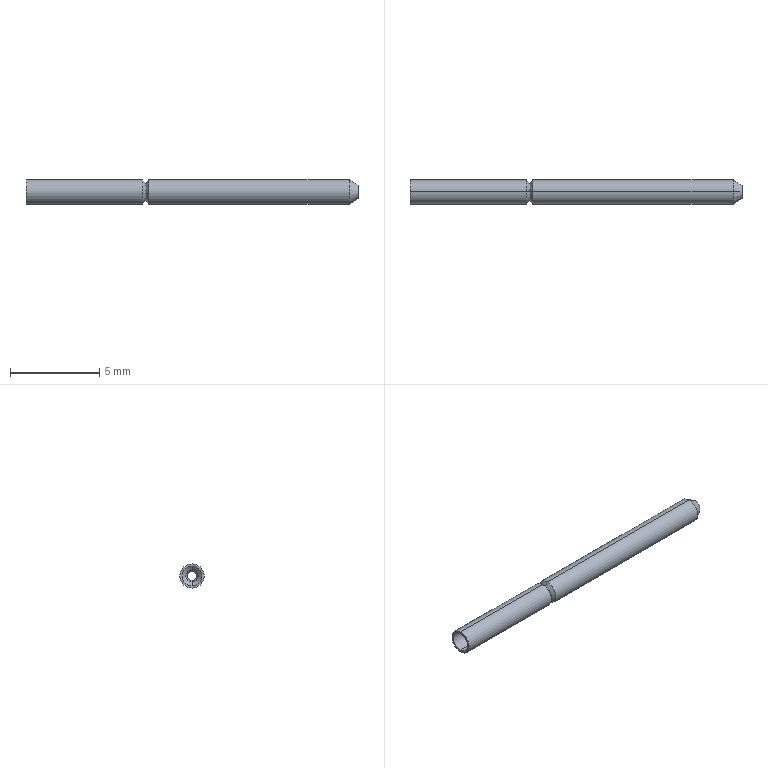Part | STEP file | Barrel_NP604_B | 1 solid | 22 faces | box 18.6 x 1.36 x 1.36 mm | volume 8.939 mm3 | cone 12 | cylinder 8 | plane 2 | commonest cylinder face diameters 1.11 x4 1.36 x4
STEP:
#1=CARTESIAN_POINT('',(6.7,0.,0.4714));
#2=VERTEX_POINT('',#1);
#3=CARTESIAN_POINT('',(6.7,0.,-0.4714));
#4=VERTEX_POINT('',#3);
#5=CARTESIAN_POINT('',(6.7,0.,0.));
#6=DIRECTION('',(-1.,0.,0.));
#7=DIRECTION('',(0.,0.,1.));
#8=AXIS2_PLACEMENT_3D('',#5,#6,#7);
#9=CIRCLE('',#8,0.4714);
#10=EDGE_CURVE('',#2,#4,#9,.T.);
#11=ORIENTED_EDGE('',*,*,#10,.T.);
#12=CARTESIAN_POINT('',(6.525,0.,-0.68));
#13=VERTEX_POINT('',#12);
#14=CARTESIAN_POINT('',(6.7,0.,-0.4714));
#15=DIRECTION('',(-0.6428,0.,-0.766));
#16=VECTOR('',#15,1000.);
#17=LINE('',#14,#16);
#18=EDGE_CURVE('',#4,#13,#17,.T.);
#19=ORIENTED_EDGE('',*,*,#18,.T.);
#20=CARTESIAN_POINT('',(6.525,0.,0.68));
#21=VERTEX_POINT('',#20);
#22=CARTESIAN_POINT('',(6.525,0.,0.));
#23=DIRECTION('',(-1.,0.,0.));
#24=DIRECTION('',(0.,0.,1.));
#25=AXIS2_PLACEMENT_3D('',#22,#23,#24);
#26=CIRCLE('',#25,0.68);
#27=EDGE_CURVE('',#21,#13,#26,.T.);
#28=ORIENTED_EDGE('',*,*,#27,.F.);
#29=CARTESIAN_POINT('',(6.7,0.,0.4714));
#30=DIRECTION('',(-0.6428,0.,0.766));
#31=VECTOR('',#30,1000.);
#32=LINE('',#29,#31);
#33=EDGE_CURVE('',#2,#21,#32,.T.);
#34=ORIENTED_EDGE('',*,*,#33,.F.);
#35=EDGE_LOOP('',(#11,#19,#28,#34));
#36=FACE_OUTER_BOUND('',#35,.T.);
#37=CARTESIAN_POINT('',(6.7,0.,0.));
#38=DIRECTION('',(-1.,0.,0.));
#39=DIRECTION('',(0.,0.,1.));
#40=AXIS2_PLACEMENT_3D('',#37,#38,#39);
#41=CONICAL_SURFACE('',#40,0.4714,0.8727);
#42=ADVANCED_FACE('',(#36),#41,.T.);
#43=ORIENTED_EDGE('',*,*,#10,.F.);
#44=CARTESIAN_POINT('',(6.875,0.,0.68));
#45=VERTEX_POINT('',#44);
#46=CARTESIAN_POINT('',(6.875,0.,0.68));
#47=DIRECTION('',(0.6428,0.,0.766));
#48=VECTOR('',#47,1000.);
#49=LINE('',#46,#48);
#50=EDGE_CURVE('',#2,#45,#49,.T.);
#51=ORIENTED_EDGE('',*,*,#50,.T.);
#52=CARTESIAN_POINT('',(6.875,0.,-0.68));
#53=VERTEX_POINT('',#52);
#54=CARTESIAN_POINT('',(6.875,0.,0.));
#55=DIRECTION('',(-1.,0.,0.));
#56=DIRECTION('',(0.,0.,1.));
#57=AXIS2_PLACEMENT_3D('',#54,#55,#56);
#58=CIRCLE('',#57,0.68);
#59=EDGE_CURVE('',#45,#53,#58,.T.);
#60=ORIENTED_EDGE('',*,*,#59,.T.);
#61=CARTESIAN_POINT('',(6.875,0.,-0.68));
#62=DIRECTION('',(0.6428,0.,-0.766));
#63=VECTOR('',#62,1000.);
#64=LINE('',#61,#63);
#65=EDGE_CURVE('',#4,#53,#64,.T.);
#66=ORIENTED_EDGE('',*,*,#65,.F.);
#67=EDGE_LOOP('',(#43,#51,#60,#66));
#68=FACE_OUTER_BOUND('',#67,.T.);
#69=CARTESIAN_POINT('',(6.875,0.,0.));
#70=DIRECTION('',(1.,0.,0.));
#71=DIRECTION('',(0.,0.,-1.));
#72=AXIS2_PLACEMENT_3D('',#69,#70,#71);
#73=CONICAL_SURFACE('',#72,0.68,0.8727);
#74=ADVANCED_FACE('',(#68),#73,.T.);
#75=CARTESIAN_POINT('',(18.1,0.,0.68));
#76=VERTEX_POINT('',#75);
#77=CARTESIAN_POINT('',(18.1,0.,-0.68));
#78=VERTEX_POINT('',#77);
#79=CARTESIAN_POINT('',(18.1,0.,0.));
#80=DIRECTION('',(-1.,0.,0.));
#81=DIRECTION('',(0.,0.,1.));
#82=AXIS2_PLACEMENT_3D('',#79,#80,#81);
#83=CIRCLE('',#82,0.68);
#84=EDGE_CURVE('',#76,#78,#83,.T.);
#85=ORIENTED_EDGE('',*,*,#84,.T.);
#86=CARTESIAN_POINT('',(18.6,0.,-0.68));
#87=DIRECTION('',(-1.,0.,0.));
#88=VECTOR('',#87,1000.);
#89=LINE('',#86,#88);
#90=EDGE_CURVE('',#78,#53,#89,.T.);
#91=ORIENTED_EDGE('',*,*,#90,.T.);
#92=ORIENTED_EDGE('',*,*,#59,.F.);
#93=CARTESIAN_POINT('',(18.6,0.,0.68));
#94=DIRECTION('',(-1.,0.,0.));
#95=VECTOR('',#94,1000.);
#96=LINE('',#93,#95);
#97=EDGE_CURVE('',#76,#45,#96,.T.);
#98=ORIENTED_EDGE('',*,*,#97,.F.);
#99=EDGE_LOOP('',(#85,#91,#92,#98));
#100=FACE_OUTER_BOUND('',#99,.T.);
#101=CARTESIAN_POINT('',(18.6,0.,0.));
#102=DIRECTION('',(-1.,0.,0.));
#103=DIRECTION('',(0.,0.,1.));
#104=AXIS2_PLACEMENT_3D('',#101,#102,#103);
#105=CYLINDRICAL_SURFACE('',#104,0.68);
#106=ADVANCED_FACE('',(#100),#105,.T.);
#107=CARTESIAN_POINT('',(18.6,0.,0.375));
#108=VERTEX_POINT('',#107);
#109=CARTESIAN_POINT('',(18.6,0.,-0.375));
#110=VERTEX_POINT('',#109);
#111=CARTESIAN_POINT('',(18.6,0.,0.));
#112=DIRECTION('',(-1.,0.,0.));
#113=DIRECTION('',(0.,0.,1.));
#114=AXIS2_PLACEMENT_3D('',#111,#112,#113);
#115=CIRCLE('',#114,0.375);
#116=EDGE_CURVE('',#108,#110,#115,.T.);
#117=ORIENTED_EDGE('',*,*,#116,.T.);
#118=CARTESIAN_POINT('',(18.6,0.,-0.375));
#119=DIRECTION('',(-0.8537,0.,-0.5208));
#120=VECTOR('',#119,1000.);
#121=LINE('',#118,#120);
#122=EDGE_CURVE('',#110,#78,#121,.T.);
#123=ORIENTED_EDGE('',*,*,#122,.T.);
#124=ORIENTED_EDGE('',*,*,#84,.F.);
#125=CARTESIAN_POINT('',(18.6,0.,0.375));
#126=DIRECTION('',(-0.8537,0.,0.5208));
#127=VECTOR('',#126,1000.);
#128=LINE('',#125,#127);
#129=EDGE_CURVE('',#108,#76,#128,.T.);
#130=ORIENTED_EDGE('',*,*,#129,.F.);
#131=EDGE_LOOP('',(#117,#123,#124,#130));
#132=FACE_OUTER_BOUND('',#131,.T.);
#133=CARTESIAN_POINT('',(18.6,0.,0.));
#134=DIRECTION('',(-1.,0.,0.));
#135=DIRECTION('',(0.,0.,1.));
#136=AXIS2_PLACEMENT_3D('',#133,#134,#135);
#137=CONICAL_SURFACE('',#136,0.375,0.5477);
#138=ADVANCED_FACE('',(#132),#137,.T.);
#139=CARTESIAN_POINT('',(18.6,0.,-0.25));
#140=VERTEX_POINT('',#139);
#141=CARTESIAN_POINT('',(18.6,0.,0.25));
#142=VERTEX_POINT('',#141);
#143=CARTESIAN_POINT('',(18.6,0.,0.));
#144=DIRECTION('',(-1.,0.,0.));
#145=DIRECTION('',(0.,0.,1.));
#146=AXIS2_PLACEMENT_3D('',#143,#144,#145);
#147=CIRCLE('',#146,0.25);
#148=EDGE_CURVE('',#140,#142,#147,.T.);
#149=ORIENTED_EDGE('',*,*,#148,.F.);
#150=CARTESIAN_POINT('',(18.1,0.,-0.555));
#151=VERTEX_POINT('',#150);
#152=CARTESIAN_POINT('',(18.1,0.,-0.555));
#153=DIRECTION('',(-0.8537,0.,-0.5208));
#154=VECTOR('',#153,1000.);
#155=LINE('',#152,#154);
#156=EDGE_CURVE('',#140,#151,#155,.T.);
#157=ORIENTED_EDGE('',*,*,#156,.T.);
#158=CARTESIAN_POINT('',(18.1,0.,0.555));
#159=VERTEX_POINT('',#158);
#160=CARTESIAN_POINT('',(18.1,0.,0.));
#161=DIRECTION('',(-1.,0.,0.));
#162=DIRECTION('',(0.,0.,1.));
#163=AXIS2_PLACEMENT_3D('',#160,#161,#162);
#164=CIRCLE('',#163,0.555);
#165=EDGE_CURVE('',#151,#159,#164,.T.);
#166=ORIENTED_EDGE('',*,*,#165,.T.);
#167=CARTESIAN_POINT('',(18.1,0.,0.555));
#168=DIRECTION('',(-0.8537,0.,0.5208));
#169=VECTOR('',#168,1000.);
#170=LINE('',#167,#169);
#171=EDGE_CURVE('',#142,#159,#170,.T.);
#172=ORIENTED_EDGE('',*,*,#171,.F.);
#173=EDGE_LOOP('',(#149,#157,#166,#172));
#174=FACE_OUTER_BOUND('',#173,.T.);
#175=CARTESIAN_POINT('',(18.1,0.,0.));
#176=DIRECTION('',(-1.,0.,0.));
#177=DIRECTION('',(0.,0.,1.));
#178=AXIS2_PLACEMENT_3D('',#175,#176,#177);
#179=CONICAL_SURFACE('',#178,0.555,0.5477);
#180=ADVANCED_FACE('',(#174),#179,.F.);
#181=ORIENTED_EDGE('',*,*,#165,.F.);
#182=CARTESIAN_POINT('',(6.88,0.,-0.555));
#183=VERTEX_POINT('',#182);
#184=CARTESIAN_POINT('',(18.6,0.,-0.555));
#185=DIRECTION('',(-1.,0.,0.));
#186=VECTOR('',#185,1000.);
#187=LINE('',#184,#186);
#188=EDGE_CURVE('',#151,#183,#187,.T.);
#189=ORIENTED_EDGE('',*,*,#188,.T.);
#190=CARTESIAN_POINT('',(6.88,0.,0.555));
#191=VERTEX_POINT('',#190);
#192=CARTESIAN_POINT('',(6.88,0.,0.));
#193=DIRECTION('',(-1.,0.,0.));
#194=DIRECTION('',(0.,0.,1.));
#195=AXIS2_PLACEMENT_3D('',#192,#193,#194);
#196=CIRCLE('',#195,0.555);
#197=EDGE_CURVE('',#183,#191,#196,.T.);
#198=ORIENTED_EDGE('',*,*,#197,.T.);
#199=CARTESIAN_POINT('',(18.6,0.,0.555));
#200=DIRECTION('',(-1.,0.,0.));
#201=VECTOR('',#200,1000.);
#202=LINE('',#199,#201);
#203=EDGE_CURVE('',#159,#191,#202,.T.);
#204=ORIENTED_EDGE('',*,*,#203,.F.);
#205=EDGE_LOOP('',(#181,#189,#198,#204));
#206=FACE_OUTER_BOUND('',#205,.T.);
#207=CARTESIAN_POINT('',(18.6,0.,0.));
#208=DIRECTION('',(-1.,0.,0.));
#209=DIRECTION('',(0.,0.,1.));
#210=AXIS2_PLACEMENT_3D('',#207,#208,#209);
#211=CYLINDRICAL_SURFACE('',#210,0.555);
#212=ADVANCED_FACE('',(#206),#211,.F.);
#213=CARTESIAN_POINT('',(6.7,0.,-0.34));
#214=VERTEX_POINT('',#213);
#215=CARTESIAN_POINT('',(6.7,0.,0.34));
#216=VERTEX_POINT('',#215);
#217=CARTESIAN_POINT('',(6.7,0.,0.));
#218=DIRECTION('',(-1.,0.,0.));
#219=DIRECTION('',(0.,0.,1.));
#220=AXIS2_PLACEMENT_3D('',#217,#218,#219);
#221=CIRCLE('',#220,0.34);
#222=EDGE_CURVE('',#214,#216,#221,.T.);
#223=ORIENTED_EDGE('',*,*,#222,.T.);
#224=CARTESIAN_POINT('',(6.7,0.,0.34));
#225=DIRECTION('',(0.6428,0.,0.766));
#226=VECTOR('',#225,1000.);
#227=LINE('',#224,#226);
#228=EDGE_CURVE('',#216,#191,#227,.T.);
#229=ORIENTED_EDGE('',*,*,#228,.T.);
#230=ORIENTED_EDGE('',*,*,#197,.F.);
#231=CARTESIAN_POINT('',(6.7,0.,-0.34));
#232=DIRECTION('',(0.6428,0.,-0.766));
#233=VECTOR('',#232,1000.);
#234=LINE('',#231,#233);
#235=EDGE_CURVE('',#214,#183,#234,.T.);
#236=ORIENTED_EDGE('',*,*,#235,.F.);
#237=EDGE_LOOP('',(#223,#229,#230,#236));
#238=FACE_OUTER_BOUND('',#237,.T.);
#239=CARTESIAN_POINT('',(6.7,0.,0.));
#240=DIRECTION('',(1.,0.,0.));
#241=DIRECTION('',(0.,0.,-1.));
#242=AXIS2_PLACEMENT_3D('',#239,#240,#241);
#243=CONICAL_SURFACE('',#242,0.34,0.8727);
#244=ADVANCED_FACE('',(#238),#243,.F.);
#245=ORIENTED_EDGE('',*,*,#222,.F.);
#246=CARTESIAN_POINT('',(6.52,0.,-0.555));
#247=VERTEX_POINT('',#246);
#248=CARTESIAN_POINT('',(6.52,0.,-0.555));
#249=DIRECTION('',(-0.6428,0.,-0.766));
#250=VECTOR('',#249,1000.);
#251=LINE('',#248,#250);
#252=EDGE_CURVE('',#214,#247,#251,.T.);
#253=ORIENTED_EDGE('',*,*,#252,.T.);
#254=CARTESIAN_POINT('',(6.52,0.,0.555));
#255=VERTEX_POINT('',#254);
#256=CARTESIAN_POINT('',(6.52,0.,0.));
#257=DIRECTION('',(-1.,0.,0.));
#258=DIRECTION('',(0.,0.,1.));
#259=AXIS2_PLACEMENT_3D('',#256,#257,#258);
#260=CIRCLE('',#259,0.555);
#261=EDGE_CURVE('',#247,#255,#260,.T.);
#262=ORIENTED_EDGE('',*,*,#261,.T.);
#263=CARTESIAN_POINT('',(6.52,0.,0.555));
#264=DIRECTION('',(-0.6428,0.,0.766));
#265=VECTOR('',#264,1000.);
#266=LINE('',#263,#265);
#267=EDGE_CURVE('',#216,#255,#266,.T.);
#268=ORIENTED_EDGE('',*,*,#267,.F.);
#269=EDGE_LOOP('',(#245,#253,#262,#268));
#270=FACE_OUTER_BOUND('',#269,.T.);
#271=CARTESIAN_POINT('',(6.52,0.,0.));
#272=DIRECTION('',(-1.,0.,0.));
#273=DIRECTION('',(0.,0.,1.));
#274=AXIS2_PLACEMENT_3D('',#271,#272,#273);
#275=CONICAL_SURFACE('',#274,0.555,0.8727);
#276=ADVANCED_FACE('',(#270),#275,.F.);
#277=ORIENTED_EDGE('',*,*,#261,.F.);
#278=CARTESIAN_POINT('',(0.,0.,-0.555));
#279=VERTEX_POINT('',#278);
#280=CARTESIAN_POINT('',(18.6,0.,-0.555));
#281=DIRECTION('',(-1.,0.,0.));
#282=VECTOR('',#281,1000.);
#283=LINE('',#280,#282);
#284=EDGE_CURVE('',#247,#279,#283,.T.);
#285=ORIENTED_EDGE('',*,*,#284,.T.);
#286=CARTESIAN_POINT('',(0.,0.,0.555));
#287=VERTEX_POINT('',#286);
#288=CARTESIAN_POINT('',(0.,0.,0.));
#289=DIRECTION('',(-1.,0.,0.));
#290=DIRECTION('',(0.,0.,1.));
#291=AXIS2_PLACEMENT_3D('',#288,#289,#290);
#292=CIRCLE('',#291,0.555);
#293=EDGE_CURVE('',#279,#287,#292,.T.);
#294=ORIENTED_EDGE('',*,*,#293,.T.);
#295=CARTESIAN_POINT('',(18.6,0.,0.555));
#296=DIRECTION('',(-1.,0.,0.));
#297=VECTOR('',#296,1000.);
#298=LINE('',#295,#297);
#299=EDGE_CURVE('',#255,#287,#298,.T.);
#300=ORIENTED_EDGE('',*,*,#299,.F.);
#301=EDGE_LOOP('',(#277,#285,#294,#300));
#302=FACE_OUTER_BOUND('',#301,.T.);
#303=CARTESIAN_POINT('',(18.6,0.,0.));
#304=DIRECTION('',(-1.,0.,0.));
#305=DIRECTION('',(0.,0.,1.));
#306=AXIS2_PLACEMENT_3D('',#303,#304,#305);
#307=CYLINDRICAL_SURFACE('',#306,0.555);
#308=ADVANCED_FACE('',(#302),#307,.F.);
#309=ORIENTED_EDGE('',*,*,#27,.T.);
#310=CARTESIAN_POINT('',(0.,0.,-0.68));
#311=VERTEX_POINT('',#310);
#312=CARTESIAN_POINT('',(18.6,0.,-0.68));
#313=DIRECTION('',(-1.,0.,0.));
#314=VECTOR('',#313,1000.);
#315=LINE('',#312,#314);
#316=EDGE_CURVE('',#13,#311,#315,.T.);
#317=ORIENTED_EDGE('',*,*,#316,.T.);
#318=CARTESIAN_POINT('',(0.,0.,0.68));
#319=VERTEX_POINT('',#318);
#320=CARTESIAN_POINT('',(0.,0.,0.));
#321=DIRECTION('',(-1.,0.,0.));
#322=DIRECTION('',(0.,0.,1.));
#323=AXIS2_PLACEMENT_3D('',#320,#321,#322);
#324=CIRCLE('',#323,0.68);
#325=EDGE_CURVE('',#319,#311,#324,.T.);
#326=ORIENTED_EDGE('',*,*,#325,.F.);
#327=CARTESIAN_POINT('',(18.6,0.,0.68));
#328=DIRECTION('',(-1.,0.,0.));
#329=VECTOR('',#328,1000.);
#330=LINE('',#327,#329);
#331=EDGE_CURVE('',#21,#319,#330,.T.);
#332=ORIENTED_EDGE('',*,*,#331,.F.);
#333=EDGE_LOOP('',(#309,#317,#326,#332));
#334=FACE_OUTER_BOUND('',#333,.T.);
#335=CARTESIAN_POINT('',(18.6,0.,0.));
#336=DIRECTION('',(-1.,0.,0.));
#337=DIRECTION('',(0.,0.,1.));
#338=AXIS2_PLACEMENT_3D('',#335,#336,#337);
#339=CYLINDRICAL_SURFACE('',#338,0.68);
#340=ADVANCED_FACE('',(#334),#339,.T.);
#341=ORIENTED_EDGE('',*,*,#316,.F.);
#342=CARTESIAN_POINT('',(6.525,0.,0.));
#343=DIRECTION('',(-1.,0.,0.));
#344=DIRECTION('',(0.,0.,1.));
#345=AXIS2_PLACEMENT_3D('',#342,#343,#344);
#346=CIRCLE('',#345,0.68);
#347=EDGE_CURVE('',#13,#21,#346,.T.);
#348=ORIENTED_EDGE('',*,*,#347,.T.);
#349=ORIENTED_EDGE('',*,*,#331,.T.);
#350=CARTESIAN_POINT('',(0.,0.,0.));
#351=DIRECTION('',(-1.,0.,0.));
#352=DIRECTION('',(0.,0.,1.));
#353=AXIS2_PLACEMENT_3D('',#350,#351,#352);
#354=CIRCLE('',#353,0.68);
#355=EDGE_CURVE('',#311,#319,#354,.T.);
#356=ORIENTED_EDGE('',*,*,#355,.F.);
#357=EDGE_LOOP('',(#341,#348,#349,#356));
#358=FACE_OUTER_BOUND('',#357,.T.);
#359=CARTESIAN_POINT('',(18.6,0.,0.));
#360=DIRECTION('',(-1.,0.,0.));
#361=DIRECTION('',(0.,0.,1.));
#362=AXIS2_PLACEMENT_3D('',#359,#360,#361);
#363=CYLINDRICAL_SURFACE('',#362,0.68);
#364=ADVANCED_FACE('',(#358),#363,.T.);
#365=CARTESIAN_POINT('',(0.,0.,0.));
#366=DIRECTION('',(-1.,0.,0.));
#367=DIRECTION('',(0.,0.,1.));
#368=AXIS2_PLACEMENT_3D('',#365,#366,#367);
#369=CIRCLE('',#368,0.555);
#370=EDGE_CURVE('',#287,#279,#369,.T.);
#371=ORIENTED_EDGE('',*,*,#370,.F.);
#372=ORIENTED_EDGE('',*,*,#293,.F.);
#373=EDGE_LOOP('',(#371,#372));
#374=FACE_BOUND('',#373,.T.);
#375=ORIENTED_EDGE('',*,*,#325,.T.);
#376=ORIENTED_EDGE('',*,*,#355,.T.);
#377=EDGE_LOOP('',(#375,#376));
#378=FACE_OUTER_BOUND('',#377,.T.);
#379=CARTESIAN_POINT('',(0.,0.68,0.));
#380=DIRECTION('',(1.,0.,0.));
#381=DIRECTION('',(0.,0.,-1.));
#382=AXIS2_PLACEMENT_3D('',#379,#380,#381);
#383=PLANE('',#382);
#384=ADVANCED_FACE('',(#374,#378),#383,.F.);
#385=ORIENTED_EDGE('',*,*,#284,.F.);
#386=CARTESIAN_POINT('',(6.52,0.,0.));
#387=DIRECTION('',(-1.,0.,0.));
#388=DIRECTION('',(0.,0.,1.));
#389=AXIS2_PLACEMENT_3D('',#386,#387,#388);
#390=CIRCLE('',#389,0.555);
#391=EDGE_CURVE('',#255,#247,#390,.T.);
#392=ORIENTED_EDGE('',*,*,#391,.F.);
#393=ORIENTED_EDGE('',*,*,#299,.T.);
#394=ORIENTED_EDGE('',*,*,#370,.T.);
#395=EDGE_LOOP('',(#385,#392,#393,#394));
#396=FACE_OUTER_BOUND('',#395,.T.);
#397=CARTESIAN_POINT('',(18.6,0.,0.));
#398=DIRECTION('',(-1.,0.,0.));
#399=DIRECTION('',(0.,0.,1.));
#400=AXIS2_PLACEMENT_3D('',#397,#398,#399);
#401=CYLINDRICAL_SURFACE('',#400,0.555);
#402=ADVANCED_FACE('',(#396),#401,.F.);
#403=ORIENTED_EDGE('',*,*,#252,.F.);
#404=CARTESIAN_POINT('',(6.7,0.,0.));
#405=DIRECTION('',(-1.,0.,0.));
#406=DIRECTION('',(0.,0.,1.));
#407=AXIS2_PLACEMENT_3D('',#404,#405,#406);
#408=CIRCLE('',#407,0.34);
#409=EDGE_CURVE('',#216,#214,#408,.T.);
#410=ORIENTED_EDGE('',*,*,#409,.F.);
#411=ORIENTED_EDGE('',*,*,#267,.T.);
#412=ORIENTED_EDGE('',*,*,#391,.T.);
#413=EDGE_LOOP('',(#403,#410,#411,#412));
#414=FACE_OUTER_BOUND('',#413,.T.);
#415=CARTESIAN_POINT('',(6.52,0.,0.));
#416=DIRECTION('',(-1.,0.,0.));
#417=DIRECTION('',(0.,0.,1.));
#418=AXIS2_PLACEMENT_3D('',#415,#416,#417);
#419=CONICAL_SURFACE('',#418,0.555,0.8727);
#420=ADVANCED_FACE('',(#414),#419,.F.);
#421=ORIENTED_EDGE('',*,*,#228,.F.);
#422=ORIENTED_EDGE('',*,*,#409,.T.);
#423=ORIENTED_EDGE('',*,*,#235,.T.);
#424=CARTESIAN_POINT('',(6.88,0.,0.));
#425=DIRECTION('',(-1.,0.,0.));
#426=DIRECTION('',(0.,0.,1.));
#427=AXIS2_PLACEMENT_3D('',#424,#425,#426);
#428=CIRCLE('',#427,0.555);
#429=EDGE_CURVE('',#191,#183,#428,.T.);
#430=ORIENTED_EDGE('',*,*,#429,.F.);
#431=EDGE_LOOP('',(#421,#422,#423,#430));
#432=FACE_OUTER_BOUND('',#431,.T.);
#433=CARTESIAN_POINT('',(6.7,0.,0.));
#434=DIRECTION('',(1.,0.,0.));
#435=DIRECTION('',(0.,0.,-1.));
#436=AXIS2_PLACEMENT_3D('',#433,#434,#435);
#437=CONICAL_SURFACE('',#436,0.34,0.8727);
#438=ADVANCED_FACE('',(#432),#437,.F.);
#439=ORIENTED_EDGE('',*,*,#188,.F.);
#440=CARTESIAN_POINT('',(18.1,0.,0.));
#441=DIRECTION('',(-1.,0.,0.));
#442=DIRECTION('',(0.,0.,1.));
#443=AXIS2_PLACEMENT_3D('',#440,#441,#442);
#444=CIRCLE('',#443,0.555);
#445=EDGE_CURVE('',#159,#151,#444,.T.);
#446=ORIENTED_EDGE('',*,*,#445,.F.);
#447=ORIENTED_EDGE('',*,*,#203,.T.);
#448=ORIENTED_EDGE('',*,*,#429,.T.);
#449=EDGE_LOOP('',(#439,#446,#447,#448));
#450=FACE_OUTER_BOUND('',#449,.T.);
#451=CARTESIAN_POINT('',(18.6,0.,0.));
#452=DIRECTION('',(-1.,0.,0.));
#453=DIRECTION('',(0.,0.,1.));
#454=AXIS2_PLACEMENT_3D('',#451,#452,#453);
#455=CYLINDRICAL_SURFACE('',#454,0.555);
#456=ADVANCED_FACE('',(#450),#455,.F.);
#457=ORIENTED_EDGE('',*,*,#156,.F.);
#458=CARTESIAN_POINT('',(18.6,0.,0.));
#459=DIRECTION('',(-1.,0.,0.));
#460=DIRECTION('',(0.,0.,1.));
#461=AXIS2_PLACEMENT_3D('',#458,#459,#460);
#462=CIRCLE('',#461,0.25);
#463=EDGE_CURVE('',#142,#140,#462,.T.);
#464=ORIENTED_EDGE('',*,*,#463,.F.);
#465=ORIENTED_EDGE('',*,*,#171,.T.);
#466=ORIENTED_EDGE('',*,*,#445,.T.);
#467=EDGE_LOOP('',(#457,#464,#465,#466));
#468=FACE_OUTER_BOUND('',#467,.T.);
#469=CARTESIAN_POINT('',(18.1,0.,0.));
#470=DIRECTION('',(-1.,0.,0.));
#471=DIRECTION('',(0.,0.,1.));
#472=AXIS2_PLACEMENT_3D('',#469,#470,#471);
#473=CONICAL_SURFACE('',#472,0.555,0.5477);
#474=ADVANCED_FACE('',(#468),#473,.F.);
#475=ORIENTED_EDGE('',*,*,#116,.F.);
#476=CARTESIAN_POINT('',(18.6,0.,0.));
#477=DIRECTION('',(-1.,0.,0.));
#478=DIRECTION('',(0.,0.,1.));
#479=AXIS2_PLACEMENT_3D('',#476,#477,#478);
#480=CIRCLE('',#479,0.375);
#481=EDGE_CURVE('',#110,#108,#480,.T.);
#482=ORIENTED_EDGE('',*,*,#481,.F.);
#483=EDGE_LOOP('',(#475,#482));
#484=FACE_OUTER_BOUND('',#483,.T.);
#485=ORIENTED_EDGE('',*,*,#463,.T.);
#486=ORIENTED_EDGE('',*,*,#148,.T.);
#487=EDGE_LOOP('',(#485,#486));
#488=FACE_BOUND('',#487,.T.);
#489=CARTESIAN_POINT('',(18.6,0.25,0.));
#490=DIRECTION('',(-1.,0.,0.));
#491=DIRECTION('',(0.,0.,1.));
#492=AXIS2_PLACEMENT_3D('',#489,#490,#491);
#493=PLANE('',#492);
#494=ADVANCED_FACE('',(#484,#488),#493,.F.);
#495=ORIENTED_EDGE('',*,*,#122,.F.);
#496=ORIENTED_EDGE('',*,*,#481,.T.);
#497=ORIENTED_EDGE('',*,*,#129,.T.);
#498=CARTESIAN_POINT('',(18.1,0.,0.));
#499=DIRECTION('',(-1.,0.,0.));
#500=DIRECTION('',(0.,0.,1.));
#501=AXIS2_PLACEMENT_3D('',#498,#499,#500);
#502=CIRCLE('',#501,0.68);
#503=EDGE_CURVE('',#78,#76,#502,.T.);
#504=ORIENTED_EDGE('',*,*,#503,.F.);
#505=EDGE_LOOP('',(#495,#496,#497,#504));
#506=FACE_OUTER_BOUND('',#505,.T.);
#507=CARTESIAN_POINT('',(18.6,0.,0.));
#508=DIRECTION('',(-1.,0.,0.));
#509=DIRECTION('',(0.,0.,1.));
#510=AXIS2_PLACEMENT_3D('',#507,#508,#509);
#511=CONICAL_SURFACE('',#510,0.375,0.5477);
#512=ADVANCED_FACE('',(#506),#511,.T.);
#513=ORIENTED_EDGE('',*,*,#90,.F.);
#514=ORIENTED_EDGE('',*,*,#503,.T.);
#515=ORIENTED_EDGE('',*,*,#97,.T.);
#516=CARTESIAN_POINT('',(6.875,0.,0.));
#517=DIRECTION('',(-1.,0.,0.));
#518=DIRECTION('',(0.,0.,1.));
#519=AXIS2_PLACEMENT_3D('',#516,#517,#518);
#520=CIRCLE('',#519,0.68);
#521=EDGE_CURVE('',#53,#45,#520,.T.);
#522=ORIENTED_EDGE('',*,*,#521,.F.);
#523=EDGE_LOOP('',(#513,#514,#515,#522));
#524=FACE_OUTER_BOUND('',#523,.T.);
#525=CARTESIAN_POINT('',(18.6,0.,0.));
#526=DIRECTION('',(-1.,0.,0.));
#527=DIRECTION('',(0.,0.,1.));
#528=AXIS2_PLACEMENT_3D('',#525,#526,#527);
#529=CYLINDRICAL_SURFACE('',#528,0.68);
#530=ADVANCED_FACE('',(#524),#529,.T.);
#531=ORIENTED_EDGE('',*,*,#50,.F.);
#532=CARTESIAN_POINT('',(6.7,0.,0.));
#533=DIRECTION('',(-1.,0.,0.));
#534=DIRECTION('',(0.,0.,1.));
#535=AXIS2_PLACEMENT_3D('',#532,#533,#534);
#536=CIRCLE('',#535,0.4714);
#537=EDGE_CURVE('',#4,#2,#536,.T.);
#538=ORIENTED_EDGE('',*,*,#537,.F.);
#539=ORIENTED_EDGE('',*,*,#65,.T.);
#540=ORIENTED_EDGE('',*,*,#521,.T.);
#541=EDGE_LOOP('',(#531,#538,#539,#540));
#542=FACE_OUTER_BOUND('',#541,.T.);
#543=CARTESIAN_POINT('',(6.875,0.,0.));
#544=DIRECTION('',(1.,0.,0.));
#545=DIRECTION('',(0.,0.,-1.));
#546=AXIS2_PLACEMENT_3D('',#543,#544,#545);
#547=CONICAL_SURFACE('',#546,0.68,0.8727);
#548=ADVANCED_FACE('',(#542),#547,.T.);
#549=ORIENTED_EDGE('',*,*,#18,.F.);
#550=ORIENTED_EDGE('',*,*,#537,.T.);
#551=ORIENTED_EDGE('',*,*,#33,.T.);
#552=ORIENTED_EDGE('',*,*,#347,.F.);
#553=EDGE_LOOP('',(#549,#550,#551,#552));
#554=FACE_OUTER_BOUND('',#553,.T.);
#555=CARTESIAN_POINT('',(6.7,0.,0.));
#556=DIRECTION('',(-1.,0.,0.));
#557=DIRECTION('',(0.,0.,1.));
#558=AXIS2_PLACEMENT_3D('',#555,#556,#557);
#559=CONICAL_SURFACE('',#558,0.4714,0.8727);
#560=ADVANCED_FACE('',(#554),#559,.T.);
#561=CLOSED_SHELL('',(#42,#74,#106,#138,#180,#212,#244,#276,#308,#340,#364,#384,#402,#420,#438,#456,#474,#494,#512,#530,#548,#560));
#562=MANIFOLD_SOLID_BREP('',#561);
#563=CARTESIAN_POINT('',(0.,0.,0.));
#564=DIRECTION('',(0.,0.,1.));
#565=DIRECTION('',(1.,0.,0.));
#566=AXIS2_PLACEMENT_3D('',#563,#564,#565);
#567=(LENGTH_UNIT()NAMED_UNIT(*)SI_UNIT(.MILLI.,.METRE.));
#568=UNCERTAINTY_MEASURE_WITH_UNIT(LENGTH_MEASURE(0.00001),#567,'','');
#569=(NAMED_UNIT(*)PLANE_ANGLE_UNIT()SI_UNIT($,.RADIAN.));
#570=(NAMED_UNIT(*)SI_UNIT($,.STERADIAN.)SOLID_ANGLE_UNIT());
#571=(GEOMETRIC_REPRESENTATION_CONTEXT(3)GLOBAL_UNCERTAINTY_ASSIGNED_CONTEXT((#568))GLOBAL_UNIT_ASSIGNED_CONTEXT((#567,#569,#570))REPRESENTATION_CONTEXT('',''));
#572=ADVANCED_BREP_SHAPE_REPRESENTATION('',(#562,#566),#571);